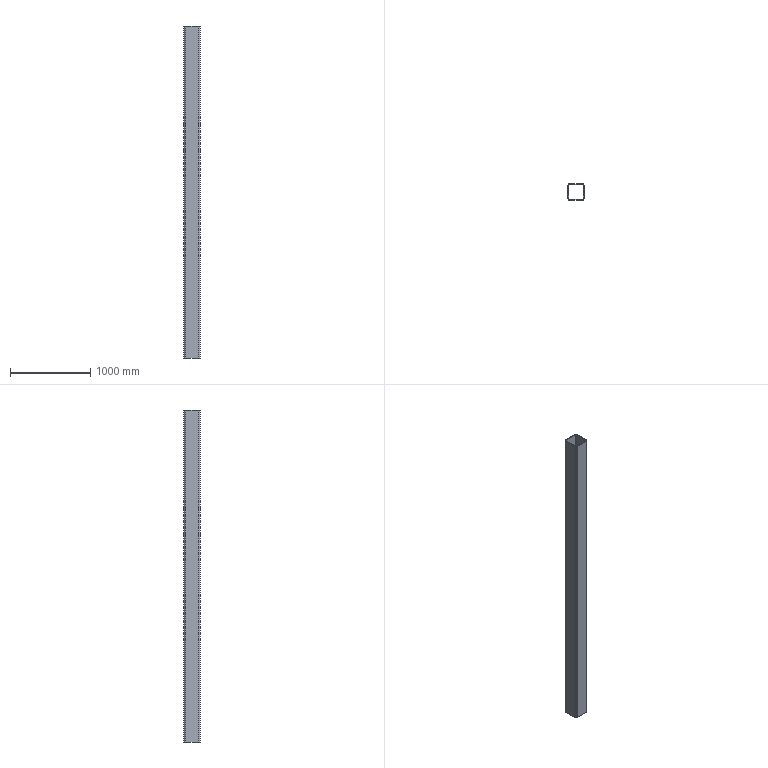Part | SolidWorks | features Extrusion 1 | 1 solid | 18 faces | box 200 x 200 x 4130 mm | volume 24467143 mm3 | plane 10 | cylinder 8 | commonest cylinder face diameters 24 x4 40 x4
STEP:
#1=CARTESIAN_POINT('',(-100.,-80.,4130.));
#2=VERTEX_POINT('',#1);
#3=CARTESIAN_POINT('',(-80.,-100.,4130.));
#4=VERTEX_POINT('',#3);
#5=CARTESIAN_POINT('',(-80.,-80.,4130.));
#6=DIRECTION('',(0.,0.,1.));
#7=DIRECTION('',(1.,0.,0.));
#8=AXIS2_PLACEMENT_3D('',#5,#6,#7);
#9=CIRCLE('',#8,20.);
#10=EDGE_CURVE('',#2,#4,#9,.T.);
#11=ORIENTED_EDGE('',*,*,#10,.T.);
#12=CARTESIAN_POINT('',(80.,-100.,4130.));
#13=VERTEX_POINT('',#12);
#14=CARTESIAN_POINT('',(-80.,-100.,4130.));
#15=DIRECTION('',(1.,0.,0.));
#16=VECTOR('',#15,1000.);
#17=LINE('',#14,#16);
#18=EDGE_CURVE('',#4,#13,#17,.T.);
#19=ORIENTED_EDGE('',*,*,#18,.T.);
#20=CARTESIAN_POINT('',(100.,-80.,4130.));
#21=VERTEX_POINT('',#20);
#22=CARTESIAN_POINT('',(80.,-80.,4130.));
#23=DIRECTION('',(0.,0.,1.));
#24=DIRECTION('',(1.,0.,0.));
#25=AXIS2_PLACEMENT_3D('',#22,#23,#24);
#26=CIRCLE('',#25,20.);
#27=EDGE_CURVE('',#13,#21,#26,.T.);
#28=ORIENTED_EDGE('',*,*,#27,.T.);
#29=CARTESIAN_POINT('',(100.,80.,4130.));
#30=VERTEX_POINT('',#29);
#31=CARTESIAN_POINT('',(100.,80.,4130.));
#32=DIRECTION('',(0.,1.,0.));
#33=VECTOR('',#32,1000.);
#34=LINE('',#31,#33);
#35=EDGE_CURVE('',#21,#30,#34,.T.);
#36=ORIENTED_EDGE('',*,*,#35,.T.);
#37=CARTESIAN_POINT('',(80.,100.,4130.));
#38=VERTEX_POINT('',#37);
#39=CARTESIAN_POINT('',(80.,80.,4130.));
#40=DIRECTION('',(0.,0.,1.));
#41=DIRECTION('',(-1.,0.,0.));
#42=AXIS2_PLACEMENT_3D('',#39,#40,#41);
#43=CIRCLE('',#42,20.);
#44=EDGE_CURVE('',#30,#38,#43,.T.);
#45=ORIENTED_EDGE('',*,*,#44,.T.);
#46=CARTESIAN_POINT('',(-80.,100.,4130.));
#47=VERTEX_POINT('',#46);
#48=CARTESIAN_POINT('',(-80.,100.,4130.));
#49=DIRECTION('',(-1.,0.,0.));
#50=VECTOR('',#49,1000.);
#51=LINE('',#48,#50);
#52=EDGE_CURVE('',#38,#47,#51,.T.);
#53=ORIENTED_EDGE('',*,*,#52,.T.);
#54=CARTESIAN_POINT('',(-100.,80.,4130.));
#55=VERTEX_POINT('',#54);
#56=CARTESIAN_POINT('',(-80.,80.,4130.));
#57=DIRECTION('',(0.,0.,1.));
#58=DIRECTION('',(1.,0.,0.));
#59=AXIS2_PLACEMENT_3D('',#56,#57,#58);
#60=CIRCLE('',#59,20.);
#61=EDGE_CURVE('',#47,#55,#60,.T.);
#62=ORIENTED_EDGE('',*,*,#61,.T.);
#63=CARTESIAN_POINT('',(-100.,80.,4130.));
#64=DIRECTION('',(0.,-1.,0.));
#65=VECTOR('',#64,1000.);
#66=LINE('',#63,#65);
#67=EDGE_CURVE('',#55,#2,#66,.T.);
#68=ORIENTED_EDGE('',*,*,#67,.T.);
#69=EDGE_LOOP('',(#11,#19,#28,#36,#45,#53,#62,#68));
#70=FACE_OUTER_BOUND('',#69,.T.);
#71=CARTESIAN_POINT('',(-92.,80.,4130.));
#72=VERTEX_POINT('',#71);
#73=CARTESIAN_POINT('',(-92.,-80.,4130.));
#74=VERTEX_POINT('',#73);
#75=CARTESIAN_POINT('',(-92.,80.,4130.));
#76=DIRECTION('',(0.,-1.,0.));
#77=VECTOR('',#76,1000.);
#78=LINE('',#75,#77);
#79=EDGE_CURVE('',#72,#74,#78,.T.);
#80=ORIENTED_EDGE('',*,*,#79,.F.);
#81=CARTESIAN_POINT('',(-80.,92.,4130.));
#82=VERTEX_POINT('',#81);
#83=CARTESIAN_POINT('',(-80.,80.,4130.));
#84=DIRECTION('',(0.,0.,1.));
#85=DIRECTION('',(1.,0.,0.));
#86=AXIS2_PLACEMENT_3D('',#83,#84,#85);
#87=CIRCLE('',#86,12.);
#88=EDGE_CURVE('',#82,#72,#87,.T.);
#89=ORIENTED_EDGE('',*,*,#88,.F.);
#90=CARTESIAN_POINT('',(80.,92.,4130.));
#91=VERTEX_POINT('',#90);
#92=CARTESIAN_POINT('',(-80.,92.,4130.));
#93=DIRECTION('',(-1.,0.,0.));
#94=VECTOR('',#93,1000.);
#95=LINE('',#92,#94);
#96=EDGE_CURVE('',#91,#82,#95,.T.);
#97=ORIENTED_EDGE('',*,*,#96,.F.);
#98=CARTESIAN_POINT('',(92.,80.,4130.));
#99=VERTEX_POINT('',#98);
#100=CARTESIAN_POINT('',(80.,80.,4130.));
#101=DIRECTION('',(0.,0.,1.));
#102=DIRECTION('',(-1.,0.,0.));
#103=AXIS2_PLACEMENT_3D('',#100,#101,#102);
#104=CIRCLE('',#103,12.);
#105=EDGE_CURVE('',#99,#91,#104,.T.);
#106=ORIENTED_EDGE('',*,*,#105,.F.);
#107=CARTESIAN_POINT('',(92.,-80.,4130.));
#108=VERTEX_POINT('',#107);
#109=CARTESIAN_POINT('',(92.,80.,4130.));
#110=DIRECTION('',(0.,1.,0.));
#111=VECTOR('',#110,1000.);
#112=LINE('',#109,#111);
#113=EDGE_CURVE('',#108,#99,#112,.T.);
#114=ORIENTED_EDGE('',*,*,#113,.F.);
#115=CARTESIAN_POINT('',(80.,-92.,4130.));
#116=VERTEX_POINT('',#115);
#117=CARTESIAN_POINT('',(80.,-80.,4130.));
#118=DIRECTION('',(0.,0.,1.));
#119=DIRECTION('',(1.,0.,0.));
#120=AXIS2_PLACEMENT_3D('',#117,#118,#119);
#121=CIRCLE('',#120,12.);
#122=EDGE_CURVE('',#116,#108,#121,.T.);
#123=ORIENTED_EDGE('',*,*,#122,.F.);
#124=CARTESIAN_POINT('',(-80.,-92.,4130.));
#125=VERTEX_POINT('',#124);
#126=CARTESIAN_POINT('',(-80.,-92.,4130.));
#127=DIRECTION('',(1.,0.,0.));
#128=VECTOR('',#127,1000.);
#129=LINE('',#126,#128);
#130=EDGE_CURVE('',#125,#116,#129,.T.);
#131=ORIENTED_EDGE('',*,*,#130,.F.);
#132=CARTESIAN_POINT('',(-80.,-80.,4130.));
#133=DIRECTION('',(0.,0.,1.));
#134=DIRECTION('',(1.,0.,0.));
#135=AXIS2_PLACEMENT_3D('',#132,#133,#134);
#136=CIRCLE('',#135,12.);
#137=EDGE_CURVE('',#74,#125,#136,.T.);
#138=ORIENTED_EDGE('',*,*,#137,.F.);
#139=EDGE_LOOP('',(#80,#89,#97,#106,#114,#123,#131,#138));
#140=FACE_BOUND('',#139,.T.);
#141=CARTESIAN_POINT('',(-80.,-80.,4130.));
#142=DIRECTION('',(0.,0.,1.));
#143=DIRECTION('',(1.,0.,0.));
#144=AXIS2_PLACEMENT_3D('',#141,#142,#143);
#145=PLANE('',#144);
#146=ADVANCED_FACE('',(#70,#140),#145,.T.);
#147=CARTESIAN_POINT('',(-100.,-80.,0.));
#148=VERTEX_POINT('',#147);
#149=CARTESIAN_POINT('',(-80.,-100.,0.));
#150=VERTEX_POINT('',#149);
#151=CARTESIAN_POINT('',(-80.,-80.,0.));
#152=DIRECTION('',(0.,0.,1.));
#153=DIRECTION('',(1.,0.,0.));
#154=AXIS2_PLACEMENT_3D('',#151,#152,#153);
#155=CIRCLE('',#154,20.);
#156=EDGE_CURVE('',#148,#150,#155,.T.);
#157=ORIENTED_EDGE('',*,*,#156,.F.);
#158=CARTESIAN_POINT('',(-100.,80.,0.));
#159=VERTEX_POINT('',#158);
#160=CARTESIAN_POINT('',(-100.,80.,0.));
#161=DIRECTION('',(0.,-1.,0.));
#162=VECTOR('',#161,1000.);
#163=LINE('',#160,#162);
#164=EDGE_CURVE('',#159,#148,#163,.T.);
#165=ORIENTED_EDGE('',*,*,#164,.F.);
#166=CARTESIAN_POINT('',(-80.,100.,0.));
#167=VERTEX_POINT('',#166);
#168=CARTESIAN_POINT('',(-80.,80.,0.));
#169=DIRECTION('',(0.,0.,1.));
#170=DIRECTION('',(1.,0.,0.));
#171=AXIS2_PLACEMENT_3D('',#168,#169,#170);
#172=CIRCLE('',#171,20.);
#173=EDGE_CURVE('',#167,#159,#172,.T.);
#174=ORIENTED_EDGE('',*,*,#173,.F.);
#175=CARTESIAN_POINT('',(80.,100.,0.));
#176=VERTEX_POINT('',#175);
#177=CARTESIAN_POINT('',(-80.,100.,0.));
#178=DIRECTION('',(-1.,0.,0.));
#179=VECTOR('',#178,1000.);
#180=LINE('',#177,#179);
#181=EDGE_CURVE('',#176,#167,#180,.T.);
#182=ORIENTED_EDGE('',*,*,#181,.F.);
#183=CARTESIAN_POINT('',(100.,80.,0.));
#184=VERTEX_POINT('',#183);
#185=CARTESIAN_POINT('',(80.,80.,0.));
#186=DIRECTION('',(0.,0.,1.));
#187=DIRECTION('',(-1.,0.,0.));
#188=AXIS2_PLACEMENT_3D('',#185,#186,#187);
#189=CIRCLE('',#188,20.);
#190=EDGE_CURVE('',#184,#176,#189,.T.);
#191=ORIENTED_EDGE('',*,*,#190,.F.);
#192=CARTESIAN_POINT('',(100.,-80.,0.));
#193=VERTEX_POINT('',#192);
#194=CARTESIAN_POINT('',(100.,80.,0.));
#195=DIRECTION('',(0.,1.,0.));
#196=VECTOR('',#195,1000.);
#197=LINE('',#194,#196);
#198=EDGE_CURVE('',#193,#184,#197,.T.);
#199=ORIENTED_EDGE('',*,*,#198,.F.);
#200=CARTESIAN_POINT('',(80.,-100.,0.));
#201=VERTEX_POINT('',#200);
#202=CARTESIAN_POINT('',(80.,-80.,0.));
#203=DIRECTION('',(0.,0.,1.));
#204=DIRECTION('',(1.,0.,0.));
#205=AXIS2_PLACEMENT_3D('',#202,#203,#204);
#206=CIRCLE('',#205,20.);
#207=EDGE_CURVE('',#201,#193,#206,.T.);
#208=ORIENTED_EDGE('',*,*,#207,.F.);
#209=CARTESIAN_POINT('',(-80.,-100.,0.));
#210=DIRECTION('',(1.,0.,0.));
#211=VECTOR('',#210,1000.);
#212=LINE('',#209,#211);
#213=EDGE_CURVE('',#150,#201,#212,.T.);
#214=ORIENTED_EDGE('',*,*,#213,.F.);
#215=EDGE_LOOP('',(#157,#165,#174,#182,#191,#199,#208,#214));
#216=FACE_OUTER_BOUND('',#215,.T.);
#217=CARTESIAN_POINT('',(-80.,92.,0.));
#218=VERTEX_POINT('',#217);
#219=CARTESIAN_POINT('',(-92.,80.,0.));
#220=VERTEX_POINT('',#219);
#221=CARTESIAN_POINT('',(-80.,80.,0.));
#222=DIRECTION('',(0.,0.,1.));
#223=DIRECTION('',(1.,0.,0.));
#224=AXIS2_PLACEMENT_3D('',#221,#222,#223);
#225=CIRCLE('',#224,12.);
#226=EDGE_CURVE('',#218,#220,#225,.T.);
#227=ORIENTED_EDGE('',*,*,#226,.T.);
#228=CARTESIAN_POINT('',(-92.,-80.,0.));
#229=VERTEX_POINT('',#228);
#230=CARTESIAN_POINT('',(-92.,80.,0.));
#231=DIRECTION('',(0.,-1.,0.));
#232=VECTOR('',#231,1000.);
#233=LINE('',#230,#232);
#234=EDGE_CURVE('',#220,#229,#233,.T.);
#235=ORIENTED_EDGE('',*,*,#234,.T.);
#236=CARTESIAN_POINT('',(-80.,-92.,0.));
#237=VERTEX_POINT('',#236);
#238=CARTESIAN_POINT('',(-80.,-80.,0.));
#239=DIRECTION('',(0.,0.,1.));
#240=DIRECTION('',(1.,0.,0.));
#241=AXIS2_PLACEMENT_3D('',#238,#239,#240);
#242=CIRCLE('',#241,12.);
#243=EDGE_CURVE('',#229,#237,#242,.T.);
#244=ORIENTED_EDGE('',*,*,#243,.T.);
#245=CARTESIAN_POINT('',(80.,-92.,0.));
#246=VERTEX_POINT('',#245);
#247=CARTESIAN_POINT('',(-80.,-92.,0.));
#248=DIRECTION('',(1.,0.,0.));
#249=VECTOR('',#248,1000.);
#250=LINE('',#247,#249);
#251=EDGE_CURVE('',#237,#246,#250,.T.);
#252=ORIENTED_EDGE('',*,*,#251,.T.);
#253=CARTESIAN_POINT('',(92.,-80.,0.));
#254=VERTEX_POINT('',#253);
#255=CARTESIAN_POINT('',(80.,-80.,0.));
#256=DIRECTION('',(0.,0.,1.));
#257=DIRECTION('',(1.,0.,0.));
#258=AXIS2_PLACEMENT_3D('',#255,#256,#257);
#259=CIRCLE('',#258,12.);
#260=EDGE_CURVE('',#246,#254,#259,.T.);
#261=ORIENTED_EDGE('',*,*,#260,.T.);
#262=CARTESIAN_POINT('',(92.,80.,0.));
#263=VERTEX_POINT('',#262);
#264=CARTESIAN_POINT('',(92.,80.,0.));
#265=DIRECTION('',(0.,1.,0.));
#266=VECTOR('',#265,1000.);
#267=LINE('',#264,#266);
#268=EDGE_CURVE('',#254,#263,#267,.T.);
#269=ORIENTED_EDGE('',*,*,#268,.T.);
#270=CARTESIAN_POINT('',(80.,92.,0.));
#271=VERTEX_POINT('',#270);
#272=CARTESIAN_POINT('',(80.,80.,0.));
#273=DIRECTION('',(0.,0.,1.));
#274=DIRECTION('',(-1.,0.,0.));
#275=AXIS2_PLACEMENT_3D('',#272,#273,#274);
#276=CIRCLE('',#275,12.);
#277=EDGE_CURVE('',#263,#271,#276,.T.);
#278=ORIENTED_EDGE('',*,*,#277,.T.);
#279=CARTESIAN_POINT('',(-80.,92.,0.));
#280=DIRECTION('',(-1.,0.,0.));
#281=VECTOR('',#280,1000.);
#282=LINE('',#279,#281);
#283=EDGE_CURVE('',#271,#218,#282,.T.);
#284=ORIENTED_EDGE('',*,*,#283,.T.);
#285=EDGE_LOOP('',(#227,#235,#244,#252,#261,#269,#278,#284));
#286=FACE_BOUND('',#285,.T.);
#287=CARTESIAN_POINT('',(-80.,-80.,0.));
#288=DIRECTION('',(0.,0.,1.));
#289=DIRECTION('',(1.,0.,0.));
#290=AXIS2_PLACEMENT_3D('',#287,#288,#289);
#291=PLANE('',#290);
#292=ADVANCED_FACE('',(#216,#286),#291,.F.);
#293=ORIENTED_EDGE('',*,*,#156,.T.);
#294=CARTESIAN_POINT('',(-80.,-100.,4130.));
#295=DIRECTION('',(0.,0.,-1.));
#296=VECTOR('',#295,1000.);
#297=LINE('',#294,#296);
#298=EDGE_CURVE('',#4,#150,#297,.T.);
#299=ORIENTED_EDGE('',*,*,#298,.F.);
#300=ORIENTED_EDGE('',*,*,#10,.F.);
#301=CARTESIAN_POINT('',(-100.,-80.,4130.));
#302=DIRECTION('',(0.,0.,-1.));
#303=VECTOR('',#302,1000.);
#304=LINE('',#301,#303);
#305=EDGE_CURVE('',#2,#148,#304,.T.);
#306=ORIENTED_EDGE('',*,*,#305,.T.);
#307=EDGE_LOOP('',(#293,#299,#300,#306));
#308=FACE_OUTER_BOUND('',#307,.T.);
#309=CARTESIAN_POINT('',(-80.,-80.,4130.));
#310=DIRECTION('',(0.,0.,-1.));
#311=DIRECTION('',(-1.,0.,0.));
#312=AXIS2_PLACEMENT_3D('',#309,#310,#311);
#313=CYLINDRICAL_SURFACE('',#312,20.);
#314=ADVANCED_FACE('',(#308),#313,.T.);
#315=ORIENTED_EDGE('',*,*,#213,.T.);
#316=CARTESIAN_POINT('',(80.,-100.,4130.));
#317=DIRECTION('',(0.,0.,-1.));
#318=VECTOR('',#317,1000.);
#319=LINE('',#316,#318);
#320=EDGE_CURVE('',#13,#201,#319,.T.);
#321=ORIENTED_EDGE('',*,*,#320,.F.);
#322=ORIENTED_EDGE('',*,*,#18,.F.);
#323=ORIENTED_EDGE('',*,*,#298,.T.);
#324=EDGE_LOOP('',(#315,#321,#322,#323));
#325=FACE_OUTER_BOUND('',#324,.T.);
#326=CARTESIAN_POINT('',(-80.,-100.,4130.));
#327=DIRECTION('',(0.,1.,0.));
#328=DIRECTION('',(0.,0.,1.));
#329=AXIS2_PLACEMENT_3D('',#326,#327,#328);
#330=PLANE('',#329);
#331=ADVANCED_FACE('',(#325),#330,.F.);
#332=ORIENTED_EDGE('',*,*,#207,.T.);
#333=CARTESIAN_POINT('',(100.,-80.,4130.));
#334=DIRECTION('',(0.,0.,-1.));
#335=VECTOR('',#334,1000.);
#336=LINE('',#333,#335);
#337=EDGE_CURVE('',#21,#193,#336,.T.);
#338=ORIENTED_EDGE('',*,*,#337,.F.);
#339=ORIENTED_EDGE('',*,*,#27,.F.);
#340=ORIENTED_EDGE('',*,*,#320,.T.);
#341=EDGE_LOOP('',(#332,#338,#339,#340));
#342=FACE_OUTER_BOUND('',#341,.T.);
#343=CARTESIAN_POINT('',(80.,-80.,4130.));
#344=DIRECTION('',(0.,0.,-1.));
#345=DIRECTION('',(-1.,0.,0.));
#346=AXIS2_PLACEMENT_3D('',#343,#344,#345);
#347=CYLINDRICAL_SURFACE('',#346,20.);
#348=ADVANCED_FACE('',(#342),#347,.T.);
#349=ORIENTED_EDGE('',*,*,#198,.T.);
#350=CARTESIAN_POINT('',(100.,80.,4130.));
#351=DIRECTION('',(0.,0.,-1.));
#352=VECTOR('',#351,1000.);
#353=LINE('',#350,#352);
#354=EDGE_CURVE('',#30,#184,#353,.T.);
#355=ORIENTED_EDGE('',*,*,#354,.F.);
#356=ORIENTED_EDGE('',*,*,#35,.F.);
#357=ORIENTED_EDGE('',*,*,#337,.T.);
#358=EDGE_LOOP('',(#349,#355,#356,#357));
#359=FACE_OUTER_BOUND('',#358,.T.);
#360=CARTESIAN_POINT('',(100.,80.,4130.));
#361=DIRECTION('',(-1.,0.,0.));
#362=DIRECTION('',(0.,-1.,0.));
#363=AXIS2_PLACEMENT_3D('',#360,#361,#362);
#364=PLANE('',#363);
#365=ADVANCED_FACE('',(#359),#364,.F.);
#366=ORIENTED_EDGE('',*,*,#190,.T.);
#367=CARTESIAN_POINT('',(80.,100.,4130.));
#368=DIRECTION('',(0.,0.,-1.));
#369=VECTOR('',#368,1000.);
#370=LINE('',#367,#369);
#371=EDGE_CURVE('',#38,#176,#370,.T.);
#372=ORIENTED_EDGE('',*,*,#371,.F.);
#373=ORIENTED_EDGE('',*,*,#44,.F.);
#374=ORIENTED_EDGE('',*,*,#354,.T.);
#375=EDGE_LOOP('',(#366,#372,#373,#374));
#376=FACE_OUTER_BOUND('',#375,.T.);
#377=CARTESIAN_POINT('',(80.,80.,4130.));
#378=DIRECTION('',(0.,0.,-1.));
#379=DIRECTION('',(-1.,0.,0.));
#380=AXIS2_PLACEMENT_3D('',#377,#378,#379);
#381=CYLINDRICAL_SURFACE('',#380,20.);
#382=ADVANCED_FACE('',(#376),#381,.T.);
#383=ORIENTED_EDGE('',*,*,#181,.T.);
#384=CARTESIAN_POINT('',(-80.,100.,4130.));
#385=DIRECTION('',(0.,0.,-1.));
#386=VECTOR('',#385,1000.);
#387=LINE('',#384,#386);
#388=EDGE_CURVE('',#47,#167,#387,.T.);
#389=ORIENTED_EDGE('',*,*,#388,.F.);
#390=ORIENTED_EDGE('',*,*,#52,.F.);
#391=ORIENTED_EDGE('',*,*,#371,.T.);
#392=EDGE_LOOP('',(#383,#389,#390,#391));
#393=FACE_OUTER_BOUND('',#392,.T.);
#394=CARTESIAN_POINT('',(-80.,100.,4130.));
#395=DIRECTION('',(0.,-1.,0.));
#396=DIRECTION('',(0.,0.,-1.));
#397=AXIS2_PLACEMENT_3D('',#394,#395,#396);
#398=PLANE('',#397);
#399=ADVANCED_FACE('',(#393),#398,.F.);
#400=ORIENTED_EDGE('',*,*,#173,.T.);
#401=CARTESIAN_POINT('',(-100.,80.,4130.));
#402=DIRECTION('',(0.,0.,-1.));
#403=VECTOR('',#402,1000.);
#404=LINE('',#401,#403);
#405=EDGE_CURVE('',#55,#159,#404,.T.);
#406=ORIENTED_EDGE('',*,*,#405,.F.);
#407=ORIENTED_EDGE('',*,*,#61,.F.);
#408=ORIENTED_EDGE('',*,*,#388,.T.);
#409=EDGE_LOOP('',(#400,#406,#407,#408));
#410=FACE_OUTER_BOUND('',#409,.T.);
#411=CARTESIAN_POINT('',(-80.,80.,4130.));
#412=DIRECTION('',(0.,0.,-1.));
#413=DIRECTION('',(-1.,0.,0.));
#414=AXIS2_PLACEMENT_3D('',#411,#412,#413);
#415=CYLINDRICAL_SURFACE('',#414,20.);
#416=ADVANCED_FACE('',(#410),#415,.T.);
#417=ORIENTED_EDGE('',*,*,#164,.T.);
#418=ORIENTED_EDGE('',*,*,#305,.F.);
#419=ORIENTED_EDGE('',*,*,#67,.F.);
#420=ORIENTED_EDGE('',*,*,#405,.T.);
#421=EDGE_LOOP('',(#417,#418,#419,#420));
#422=FACE_OUTER_BOUND('',#421,.T.);
#423=CARTESIAN_POINT('',(-100.,80.,4130.));
#424=DIRECTION('',(1.,0.,0.));
#425=DIRECTION('',(0.,1.,0.));
#426=AXIS2_PLACEMENT_3D('',#423,#424,#425);
#427=PLANE('',#426);
#428=ADVANCED_FACE('',(#422),#427,.F.);
#429=ORIENTED_EDGE('',*,*,#226,.F.);
#430=CARTESIAN_POINT('',(-80.,92.,4130.));
#431=DIRECTION('',(0.,0.,-1.));
#432=VECTOR('',#431,1000.);
#433=LINE('',#430,#432);
#434=EDGE_CURVE('',#82,#218,#433,.T.);
#435=ORIENTED_EDGE('',*,*,#434,.F.);
#436=ORIENTED_EDGE('',*,*,#88,.T.);
#437=CARTESIAN_POINT('',(-92.,80.,4130.));
#438=DIRECTION('',(0.,0.,-1.));
#439=VECTOR('',#438,1000.);
#440=LINE('',#437,#439);
#441=EDGE_CURVE('',#72,#220,#440,.T.);
#442=ORIENTED_EDGE('',*,*,#441,.T.);
#443=EDGE_LOOP('',(#429,#435,#436,#442));
#444=FACE_OUTER_BOUND('',#443,.T.);
#445=CARTESIAN_POINT('',(-80.,80.,4130.));
#446=DIRECTION('',(0.,0.,-1.));
#447=DIRECTION('',(-1.,0.,0.));
#448=AXIS2_PLACEMENT_3D('',#445,#446,#447);
#449=CYLINDRICAL_SURFACE('',#448,12.);
#450=ADVANCED_FACE('',(#444),#449,.F.);
#451=ORIENTED_EDGE('',*,*,#234,.F.);
#452=ORIENTED_EDGE('',*,*,#441,.F.);
#453=ORIENTED_EDGE('',*,*,#79,.T.);
#454=CARTESIAN_POINT('',(-92.,-80.,4130.));
#455=DIRECTION('',(0.,0.,-1.));
#456=VECTOR('',#455,1000.);
#457=LINE('',#454,#456);
#458=EDGE_CURVE('',#74,#229,#457,.T.);
#459=ORIENTED_EDGE('',*,*,#458,.T.);
#460=EDGE_LOOP('',(#451,#452,#453,#459));
#461=FACE_OUTER_BOUND('',#460,.T.);
#462=CARTESIAN_POINT('',(-92.,80.,4130.));
#463=DIRECTION('',(1.,0.,0.));
#464=DIRECTION('',(0.,0.,-1.));
#465=AXIS2_PLACEMENT_3D('',#462,#463,#464);
#466=PLANE('',#465);
#467=ADVANCED_FACE('',(#461),#466,.T.);
#468=ORIENTED_EDGE('',*,*,#243,.F.);
#469=ORIENTED_EDGE('',*,*,#458,.F.);
#470=ORIENTED_EDGE('',*,*,#137,.T.);
#471=CARTESIAN_POINT('',(-80.,-92.,4130.));
#472=DIRECTION('',(0.,0.,-1.));
#473=VECTOR('',#472,1000.);
#474=LINE('',#471,#473);
#475=EDGE_CURVE('',#125,#237,#474,.T.);
#476=ORIENTED_EDGE('',*,*,#475,.T.);
#477=EDGE_LOOP('',(#468,#469,#470,#476));
#478=FACE_OUTER_BOUND('',#477,.T.);
#479=CARTESIAN_POINT('',(-80.,-80.,4130.));
#480=DIRECTION('',(0.,0.,-1.));
#481=DIRECTION('',(-1.,0.,0.));
#482=AXIS2_PLACEMENT_3D('',#479,#480,#481);
#483=CYLINDRICAL_SURFACE('',#482,12.);
#484=ADVANCED_FACE('',(#478),#483,.F.);
#485=ORIENTED_EDGE('',*,*,#251,.F.);
#486=ORIENTED_EDGE('',*,*,#475,.F.);
#487=ORIENTED_EDGE('',*,*,#130,.T.);
#488=CARTESIAN_POINT('',(80.,-92.,4130.));
#489=DIRECTION('',(0.,0.,-1.));
#490=VECTOR('',#489,1000.);
#491=LINE('',#488,#490);
#492=EDGE_CURVE('',#116,#246,#491,.T.);
#493=ORIENTED_EDGE('',*,*,#492,.T.);
#494=EDGE_LOOP('',(#485,#486,#487,#493));
#495=FACE_OUTER_BOUND('',#494,.T.);
#496=CARTESIAN_POINT('',(-80.,-92.,4130.));
#497=DIRECTION('',(0.,1.,0.));
#498=DIRECTION('',(0.,0.,1.));
#499=AXIS2_PLACEMENT_3D('',#496,#497,#498);
#500=PLANE('',#499);
#501=ADVANCED_FACE('',(#495),#500,.T.);
#502=ORIENTED_EDGE('',*,*,#260,.F.);
#503=ORIENTED_EDGE('',*,*,#492,.F.);
#504=ORIENTED_EDGE('',*,*,#122,.T.);
#505=CARTESIAN_POINT('',(92.,-80.,4130.));
#506=DIRECTION('',(0.,0.,-1.));
#507=VECTOR('',#506,1000.);
#508=LINE('',#505,#507);
#509=EDGE_CURVE('',#108,#254,#508,.T.);
#510=ORIENTED_EDGE('',*,*,#509,.T.);
#511=EDGE_LOOP('',(#502,#503,#504,#510));
#512=FACE_OUTER_BOUND('',#511,.T.);
#513=CARTESIAN_POINT('',(80.,-80.,4130.));
#514=DIRECTION('',(0.,0.,-1.));
#515=DIRECTION('',(-1.,0.,0.));
#516=AXIS2_PLACEMENT_3D('',#513,#514,#515);
#517=CYLINDRICAL_SURFACE('',#516,12.);
#518=ADVANCED_FACE('',(#512),#517,.F.);
#519=ORIENTED_EDGE('',*,*,#268,.F.);
#520=ORIENTED_EDGE('',*,*,#509,.F.);
#521=ORIENTED_EDGE('',*,*,#113,.T.);
#522=CARTESIAN_POINT('',(92.,80.,4130.));
#523=DIRECTION('',(0.,0.,-1.));
#524=VECTOR('',#523,1000.);
#525=LINE('',#522,#524);
#526=EDGE_CURVE('',#99,#263,#525,.T.);
#527=ORIENTED_EDGE('',*,*,#526,.T.);
#528=EDGE_LOOP('',(#519,#520,#521,#527));
#529=FACE_OUTER_BOUND('',#528,.T.);
#530=CARTESIAN_POINT('',(92.,80.,4130.));
#531=DIRECTION('',(-1.,0.,0.));
#532=DIRECTION('',(0.,-1.,0.));
#533=AXIS2_PLACEMENT_3D('',#530,#531,#532);
#534=PLANE('',#533);
#535=ADVANCED_FACE('',(#529),#534,.T.);
#536=ORIENTED_EDGE('',*,*,#277,.F.);
#537=ORIENTED_EDGE('',*,*,#526,.F.);
#538=ORIENTED_EDGE('',*,*,#105,.T.);
#539=CARTESIAN_POINT('',(80.,92.,4130.));
#540=DIRECTION('',(0.,0.,-1.));
#541=VECTOR('',#540,1000.);
#542=LINE('',#539,#541);
#543=EDGE_CURVE('',#91,#271,#542,.T.);
#544=ORIENTED_EDGE('',*,*,#543,.T.);
#545=EDGE_LOOP('',(#536,#537,#538,#544));
#546=FACE_OUTER_BOUND('',#545,.T.);
#547=CARTESIAN_POINT('',(80.,80.,4130.));
#548=DIRECTION('',(0.,0.,-1.));
#549=DIRECTION('',(-1.,0.,0.));
#550=AXIS2_PLACEMENT_3D('',#547,#548,#549);
#551=CYLINDRICAL_SURFACE('',#550,12.);
#552=ADVANCED_FACE('',(#546),#551,.F.);
#553=ORIENTED_EDGE('',*,*,#283,.F.);
#554=ORIENTED_EDGE('',*,*,#543,.F.);
#555=ORIENTED_EDGE('',*,*,#96,.T.);
#556=ORIENTED_EDGE('',*,*,#434,.T.);
#557=EDGE_LOOP('',(#553,#554,#555,#556));
#558=FACE_OUTER_BOUND('',#557,.T.);
#559=CARTESIAN_POINT('',(-80.,92.,4130.));
#560=DIRECTION('',(0.,-1.,0.));
#561=DIRECTION('',(0.,0.,-1.));
#562=AXIS2_PLACEMENT_3D('',#559,#560,#561);
#563=PLANE('',#562);
#564=ADVANCED_FACE('',(#558),#563,.T.);
#565=CLOSED_SHELL('',(#146,#292,#314,#331,#348,#365,#382,#399,#416,#428,#450,#467,#484,#501,#518,#535,#552,#564));
#566=MANIFOLD_SOLID_BREP('',#565);
#567=CARTESIAN_POINT('',(0.,0.,0.));
#568=DIRECTION('',(0.,0.,1.));
#569=DIRECTION('',(1.,0.,0.));
#570=AXIS2_PLACEMENT_3D('',#567,#568,#569);
#571=(LENGTH_UNIT()NAMED_UNIT(*)SI_UNIT(.MILLI.,.METRE.));
#572=UNCERTAINTY_MEASURE_WITH_UNIT(LENGTH_MEASURE(0.00001),#571,'','');
#573=(NAMED_UNIT(*)PLANE_ANGLE_UNIT()SI_UNIT($,.RADIAN.));
#574=(NAMED_UNIT(*)SI_UNIT($,.STERADIAN.)SOLID_ANGLE_UNIT());
#575=(GEOMETRIC_REPRESENTATION_CONTEXT(3)GLOBAL_UNCERTAINTY_ASSIGNED_CONTEXT((#572))GLOBAL_UNIT_ASSIGNED_CONTEXT((#571,#573,#574))REPRESENTATION_CONTEXT('',''));
#576=ADVANCED_BREP_SHAPE_REPRESENTATION('',(#566,#570),#575);